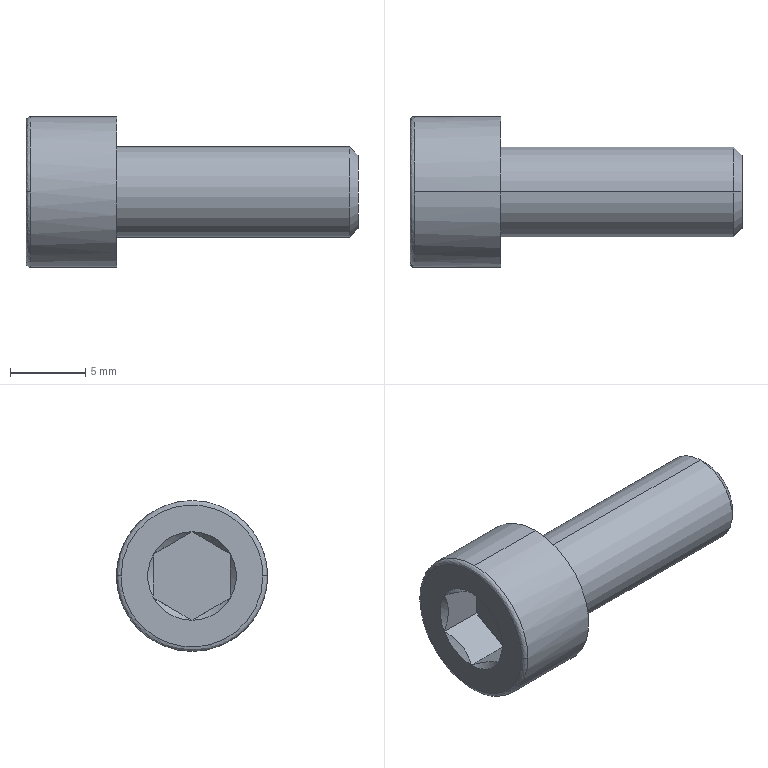Part | SolidWorks | features BaseBody 1 | 1 solid | 24 faces | box 22 x 10 x 10 mm | volume 852.514 mm3 | plane 10 | cone 8 | cylinder 4 | spline 2 | commonest cylinder face diameters 6 x2 10 x2
STEP:
#1=CARTESIAN_POINT('',(225.547,1059.506,-452.345));
#2=VERTEX_POINT('',#1);
#3=CARTESIAN_POINT('',(225.547,1050.106,-452.345));
#4=VERTEX_POINT('',#3);
#5=CARTESIAN_POINT('',(225.547,1059.506,-452.345));
#6=CARTESIAN_POINT('',(225.547,1059.506,-442.945));
#7=CARTESIAN_POINT('',(225.547,1050.106,-442.945));
#8=CARTESIAN_POINT('',(225.547,1050.106,-452.345));
#9=(BOUNDED_CURVE()B_SPLINE_CURVE(3,(#5,#6,#7,#8),.UNSPECIFIED.,.F.,.F.)B_SPLINE_CURVE_WITH_KNOTS((4,4),(0.,1.),.UNSPECIFIED.)CURVE()GEOMETRIC_REPRESENTATION_ITEM()RATIONAL_B_SPLINE_CURVE((1.,0.3333,0.3333,1.))REPRESENTATION_ITEM(''));
#10=EDGE_CURVE('',#2,#4,#9,.T.);
#11=ORIENTED_EDGE('',*,*,#10,.T.);
#12=CARTESIAN_POINT('',(225.847,1049.806,-452.345));
#13=VERTEX_POINT('',#12);
#14=CARTESIAN_POINT('',(225.847,1050.106,-452.345));
#15=DIRECTION('',(0.,0.,1.));
#16=DIRECTION('',(0.,-1.,0.));
#17=AXIS2_PLACEMENT_3D('',#14,#15,#16);
#18=CIRCLE('',#17,0.3);
#19=EDGE_CURVE('',#4,#13,#18,.T.);
#20=ORIENTED_EDGE('',*,*,#19,.T.);
#21=CARTESIAN_POINT('',(225.847,1054.806,-447.345));
#22=VERTEX_POINT('',#21);
#23=CARTESIAN_POINT('',(225.847,1054.806,-452.345));
#24=DIRECTION('',(1.,0.,0.));
#25=DIRECTION('',(0.,0.,-1.));
#26=AXIS2_PLACEMENT_3D('',#23,#24,#25);
#27=CIRCLE('',#26,5.);
#28=EDGE_CURVE('',#22,#13,#27,.T.);
#29=ORIENTED_EDGE('',*,*,#28,.F.);
#30=CARTESIAN_POINT('',(225.847,1059.806,-452.345));
#31=VERTEX_POINT('',#30);
#32=CARTESIAN_POINT('',(225.847,1054.806,-452.345));
#33=DIRECTION('',(1.,0.,0.));
#34=DIRECTION('',(0.,0.,-1.));
#35=AXIS2_PLACEMENT_3D('',#32,#33,#34);
#36=CIRCLE('',#35,5.);
#37=EDGE_CURVE('',#31,#22,#36,.T.);
#38=ORIENTED_EDGE('',*,*,#37,.F.);
#39=CARTESIAN_POINT('',(225.847,1059.506,-452.345));
#40=DIRECTION('',(0.,0.,-1.));
#41=DIRECTION('',(0.,1.,0.));
#42=AXIS2_PLACEMENT_3D('',#39,#40,#41);
#43=CIRCLE('',#42,0.3);
#44=EDGE_CURVE('',#2,#31,#43,.T.);
#45=ORIENTED_EDGE('',*,*,#44,.F.);
#46=EDGE_LOOP('',(#11,#20,#29,#38,#45));
#47=FACE_OUTER_BOUND('',#46,.T.);
#48=CARTESIAN_POINT('',(225.547,1050.106,-452.345));
#49=CARTESIAN_POINT('',(225.547,1050.106,-442.945));
#50=CARTESIAN_POINT('',(225.547,1059.506,-442.945));
#51=CARTESIAN_POINT('',(225.547,1059.506,-452.345));
#52=CARTESIAN_POINT('',(225.547,1049.93,-452.345));
#53=CARTESIAN_POINT('',(225.547,1049.93,-442.593));
#54=CARTESIAN_POINT('',(225.547,1059.681,-442.593));
#55=CARTESIAN_POINT('',(225.547,1059.681,-452.345));
#56=CARTESIAN_POINT('',(225.671,1049.806,-452.345));
#57=CARTESIAN_POINT('',(225.671,1049.806,-442.345));
#58=CARTESIAN_POINT('',(225.671,1059.806,-442.345));
#59=CARTESIAN_POINT('',(225.671,1059.806,-452.345));
#60=CARTESIAN_POINT('',(225.847,1049.806,-452.345));
#61=CARTESIAN_POINT('',(225.847,1049.806,-442.345));
#62=CARTESIAN_POINT('',(225.847,1059.806,-442.345));
#63=CARTESIAN_POINT('',(225.847,1059.806,-452.345));
#64=(BOUNDED_SURFACE()B_SPLINE_SURFACE(3,3,((#48,#49,#50,#51),(#52,#53,#54,#55),(#56,#57,#58,#59),(#60,#61,#62,#63)),.UNSPECIFIED.,.F.,.F.,.F.)B_SPLINE_SURFACE_WITH_KNOTS((4,4),(4,4),(0.,1.),(0.,1.),.UNSPECIFIED.)GEOMETRIC_REPRESENTATION_ITEM()RATIONAL_B_SPLINE_SURFACE(((1.,0.3333,0.3333,1.),(0.8047,0.2682,0.2682,0.8047),(0.8047,0.2682,0.2682,0.8047),(1.,0.3333,0.3333,1.)))REPRESENTATION_ITEM('')SURFACE());
#65=ADVANCED_FACE('',(#47),#64,.T.);
#66=CARTESIAN_POINT('',(246.992,1054.806,-449.345));
#67=VERTEX_POINT('',#66);
#68=CARTESIAN_POINT('',(246.992,1054.806,-455.345));
#69=VERTEX_POINT('',#68);
#70=CARTESIAN_POINT('',(246.992,1054.806,-452.345));
#71=DIRECTION('',(-1.,0.,0.));
#72=DIRECTION('',(0.,0.,1.));
#73=AXIS2_PLACEMENT_3D('',#70,#71,#72);
#74=CIRCLE('',#73,3.);
#75=EDGE_CURVE('',#67,#69,#74,.T.);
#76=ORIENTED_EDGE('',*,*,#75,.T.);
#77=CARTESIAN_POINT('',(231.547,1054.806,-455.345));
#78=VERTEX_POINT('',#77);
#79=CARTESIAN_POINT('',(247.547,1054.806,-455.345));
#80=DIRECTION('',(-1.,0.,0.));
#81=VECTOR('',#80,1000.);
#82=LINE('',#79,#81);
#83=EDGE_CURVE('',#69,#78,#82,.T.);
#84=ORIENTED_EDGE('',*,*,#83,.T.);
#85=CARTESIAN_POINT('',(231.547,1054.806,-449.345));
#86=VERTEX_POINT('',#85);
#87=CARTESIAN_POINT('',(231.547,1054.806,-452.345));
#88=DIRECTION('',(1.,0.,0.));
#89=DIRECTION('',(0.,0.,1.));
#90=AXIS2_PLACEMENT_3D('',#87,#88,#89);
#91=CIRCLE('',#90,3.);
#92=EDGE_CURVE('',#78,#86,#91,.T.);
#93=ORIENTED_EDGE('',*,*,#92,.T.);
#94=CARTESIAN_POINT('',(247.547,1054.806,-449.345));
#95=DIRECTION('',(-1.,0.,0.));
#96=VECTOR('',#95,1000.);
#97=LINE('',#94,#96);
#98=EDGE_CURVE('',#67,#86,#97,.T.);
#99=ORIENTED_EDGE('',*,*,#98,.F.);
#100=EDGE_LOOP('',(#76,#84,#93,#99));
#101=FACE_OUTER_BOUND('',#100,.T.);
#102=CARTESIAN_POINT('',(247.547,1054.806,-452.345));
#103=DIRECTION('',(-1.,0.,0.));
#104=DIRECTION('',(0.,0.,1.));
#105=AXIS2_PLACEMENT_3D('',#102,#103,#104);
#106=CYLINDRICAL_SURFACE('',#105,3.);
#107=ADVANCED_FACE('',(#101),#106,.T.);
#108=CARTESIAN_POINT('',(247.547,1054.806,-449.9));
#109=VERTEX_POINT('',#108);
#110=CARTESIAN_POINT('',(247.547,1054.806,-454.79));
#111=VERTEX_POINT('',#110);
#112=CARTESIAN_POINT('',(247.547,1054.806,-452.345));
#113=DIRECTION('',(-1.,0.,0.));
#114=DIRECTION('',(0.,0.,1.));
#115=AXIS2_PLACEMENT_3D('',#112,#113,#114);
#116=CIRCLE('',#115,2.445);
#117=EDGE_CURVE('',#109,#111,#116,.T.);
#118=ORIENTED_EDGE('',*,*,#117,.T.);
#119=CARTESIAN_POINT('',(246.992,1054.806,-455.345));
#120=DIRECTION('',(-0.7071,0.,-0.7071));
#121=VECTOR('',#120,1000.);
#122=LINE('',#119,#121);
#123=EDGE_CURVE('',#111,#69,#122,.T.);
#124=ORIENTED_EDGE('',*,*,#123,.T.);
#125=ORIENTED_EDGE('',*,*,#75,.F.);
#126=CARTESIAN_POINT('',(246.992,1054.806,-449.345));
#127=DIRECTION('',(-0.7071,0.,0.7071));
#128=VECTOR('',#127,1000.);
#129=LINE('',#126,#128);
#130=EDGE_CURVE('',#109,#67,#129,.T.);
#131=ORIENTED_EDGE('',*,*,#130,.F.);
#132=EDGE_LOOP('',(#118,#124,#125,#131));
#133=FACE_OUTER_BOUND('',#132,.T.);
#134=CARTESIAN_POINT('',(246.992,1054.806,-452.345));
#135=DIRECTION('',(-1.,0.,0.));
#136=DIRECTION('',(0.,0.,1.));
#137=AXIS2_PLACEMENT_3D('',#134,#135,#136);
#138=CONICAL_SURFACE('',#137,3.,0.7854);
#139=ADVANCED_FACE('',(#133),#138,.T.);
#140=CARTESIAN_POINT('',(225.847,1054.806,-457.345));
#141=VERTEX_POINT('',#140);
#142=CARTESIAN_POINT('',(225.847,1054.806,-452.345));
#143=DIRECTION('',(1.,0.,0.));
#144=DIRECTION('',(0.,0.,-1.));
#145=AXIS2_PLACEMENT_3D('',#142,#143,#144);
#146=CIRCLE('',#145,5.);
#147=EDGE_CURVE('',#141,#31,#146,.T.);
#148=ORIENTED_EDGE('',*,*,#147,.T.);
#149=ORIENTED_EDGE('',*,*,#37,.T.);
#150=CARTESIAN_POINT('',(231.547,1054.806,-447.345));
#151=VERTEX_POINT('',#150);
#152=CARTESIAN_POINT('',(225.547,1054.806,-447.345));
#153=DIRECTION('',(1.,0.,0.));
#154=VECTOR('',#153,1000.);
#155=LINE('',#152,#154);
#156=EDGE_CURVE('',#22,#151,#155,.T.);
#157=ORIENTED_EDGE('',*,*,#156,.T.);
#158=CARTESIAN_POINT('',(231.547,1054.806,-457.345));
#159=VERTEX_POINT('',#158);
#160=CARTESIAN_POINT('',(231.547,1054.806,-452.345));
#161=DIRECTION('',(-1.,0.,0.));
#162=DIRECTION('',(0.,0.,-1.));
#163=AXIS2_PLACEMENT_3D('',#160,#161,#162);
#164=CIRCLE('',#163,5.);
#165=EDGE_CURVE('',#151,#159,#164,.T.);
#166=ORIENTED_EDGE('',*,*,#165,.T.);
#167=CARTESIAN_POINT('',(225.547,1054.806,-457.345));
#168=DIRECTION('',(1.,0.,0.));
#169=VECTOR('',#168,1000.);
#170=LINE('',#167,#169);
#171=EDGE_CURVE('',#141,#159,#170,.T.);
#172=ORIENTED_EDGE('',*,*,#171,.F.);
#173=EDGE_LOOP('',(#148,#149,#157,#166,#172));
#174=FACE_OUTER_BOUND('',#173,.T.);
#175=CARTESIAN_POINT('',(225.547,1054.806,-452.345));
#176=DIRECTION('',(1.,0.,0.));
#177=DIRECTION('',(0.,0.,-1.));
#178=AXIS2_PLACEMENT_3D('',#175,#176,#177);
#179=CYLINDRICAL_SURFACE('',#178,5.);
#180=ADVANCED_FACE('',(#174),#179,.T.);
#181=ORIENTED_EDGE('',*,*,#83,.F.);
#182=CARTESIAN_POINT('',(246.992,1054.806,-452.345));
#183=DIRECTION('',(-1.,0.,0.));
#184=DIRECTION('',(0.,0.,1.));
#185=AXIS2_PLACEMENT_3D('',#182,#183,#184);
#186=CIRCLE('',#185,3.);
#187=EDGE_CURVE('',#69,#67,#186,.T.);
#188=ORIENTED_EDGE('',*,*,#187,.T.);
#189=ORIENTED_EDGE('',*,*,#98,.T.);
#190=CARTESIAN_POINT('',(231.547,1054.806,-452.345));
#191=DIRECTION('',(1.,0.,0.));
#192=DIRECTION('',(0.,0.,1.));
#193=AXIS2_PLACEMENT_3D('',#190,#191,#192);
#194=CIRCLE('',#193,3.);
#195=EDGE_CURVE('',#86,#78,#194,.T.);
#196=ORIENTED_EDGE('',*,*,#195,.T.);
#197=EDGE_LOOP('',(#181,#188,#189,#196));
#198=FACE_OUTER_BOUND('',#197,.T.);
#199=CARTESIAN_POINT('',(247.547,1054.806,-452.345));
#200=DIRECTION('',(-1.,0.,0.));
#201=DIRECTION('',(0.,0.,1.));
#202=AXIS2_PLACEMENT_3D('',#199,#200,#201);
#203=CYLINDRICAL_SURFACE('',#202,3.);
#204=ADVANCED_FACE('',(#198),#203,.T.);
#205=ORIENTED_EDGE('',*,*,#123,.F.);
#206=CARTESIAN_POINT('',(247.547,1054.806,-452.345));
#207=DIRECTION('',(-1.,0.,0.));
#208=DIRECTION('',(0.,0.,1.));
#209=AXIS2_PLACEMENT_3D('',#206,#207,#208);
#210=CIRCLE('',#209,2.445);
#211=EDGE_CURVE('',#111,#109,#210,.T.);
#212=ORIENTED_EDGE('',*,*,#211,.T.);
#213=ORIENTED_EDGE('',*,*,#130,.T.);
#214=ORIENTED_EDGE('',*,*,#187,.F.);
#215=EDGE_LOOP('',(#205,#212,#213,#214));
#216=FACE_OUTER_BOUND('',#215,.T.);
#217=CARTESIAN_POINT('',(246.992,1054.806,-452.345));
#218=DIRECTION('',(-1.,0.,0.));
#219=DIRECTION('',(0.,0.,1.));
#220=AXIS2_PLACEMENT_3D('',#217,#218,#219);
#221=CONICAL_SURFACE('',#220,3.,0.7854);
#222=ADVANCED_FACE('',(#216),#221,.T.);
#223=ORIENTED_EDGE('',*,*,#195,.F.);
#224=ORIENTED_EDGE('',*,*,#92,.F.);
#225=EDGE_LOOP('',(#223,#224));
#226=FACE_BOUND('',#225,.T.);
#227=CARTESIAN_POINT('',(231.547,1054.806,-452.345));
#228=DIRECTION('',(-1.,0.,0.));
#229=DIRECTION('',(0.,0.,-1.));
#230=AXIS2_PLACEMENT_3D('',#227,#228,#229);
#231=CIRCLE('',#230,5.);
#232=EDGE_CURVE('',#159,#151,#231,.T.);
#233=ORIENTED_EDGE('',*,*,#232,.F.);
#234=ORIENTED_EDGE('',*,*,#165,.F.);
#235=EDGE_LOOP('',(#233,#234));
#236=FACE_OUTER_BOUND('',#235,.T.);
#237=CARTESIAN_POINT('',(231.547,1054.806,-452.345));
#238=DIRECTION('',(-1.,0.,0.));
#239=DIRECTION('',(0.,0.,1.));
#240=AXIS2_PLACEMENT_3D('',#237,#238,#239);
#241=PLANE('',#240);
#242=ADVANCED_FACE('',(#226,#236),#241,.F.);
#243=ORIENTED_EDGE('',*,*,#117,.F.);
#244=ORIENTED_EDGE('',*,*,#211,.F.);
#245=EDGE_LOOP('',(#243,#244));
#246=FACE_OUTER_BOUND('',#245,.T.);
#247=CARTESIAN_POINT('',(247.547,1054.806,-452.345));
#248=DIRECTION('',(1.,0.,0.));
#249=DIRECTION('',(0.,0.,-1.));
#250=AXIS2_PLACEMENT_3D('',#247,#248,#249);
#251=PLANE('',#250);
#252=ADVANCED_FACE('',(#246),#251,.T.);
#253=ORIENTED_EDGE('',*,*,#156,.F.);
#254=ORIENTED_EDGE('',*,*,#28,.T.);
#255=CARTESIAN_POINT('',(225.847,1054.806,-452.345));
#256=DIRECTION('',(1.,0.,0.));
#257=DIRECTION('',(0.,0.,-1.));
#258=AXIS2_PLACEMENT_3D('',#255,#256,#257);
#259=CIRCLE('',#258,5.);
#260=EDGE_CURVE('',#13,#141,#259,.T.);
#261=ORIENTED_EDGE('',*,*,#260,.T.);
#262=ORIENTED_EDGE('',*,*,#171,.T.);
#263=ORIENTED_EDGE('',*,*,#232,.T.);
#264=EDGE_LOOP('',(#253,#254,#261,#262,#263));
#265=FACE_OUTER_BOUND('',#264,.T.);
#266=CARTESIAN_POINT('',(225.547,1054.806,-452.345));
#267=DIRECTION('',(1.,0.,0.));
#268=DIRECTION('',(0.,0.,-1.));
#269=AXIS2_PLACEMENT_3D('',#266,#267,#268);
#270=CYLINDRICAL_SURFACE('',#269,5.);
#271=ADVANCED_FACE('',(#265),#270,.T.);
#272=ORIENTED_EDGE('',*,*,#19,.F.);
#273=CARTESIAN_POINT('',(225.547,1050.106,-452.345));
#274=CARTESIAN_POINT('',(225.547,1050.106,-461.745));
#275=CARTESIAN_POINT('',(225.547,1059.506,-461.745));
#276=CARTESIAN_POINT('',(225.547,1059.506,-452.345));
#277=(BOUNDED_CURVE()B_SPLINE_CURVE(3,(#273,#274,#275,#276),.UNSPECIFIED.,.F.,.F.)B_SPLINE_CURVE_WITH_KNOTS((4,4),(0.,1.),.UNSPECIFIED.)CURVE()GEOMETRIC_REPRESENTATION_ITEM()RATIONAL_B_SPLINE_CURVE((1.,0.3333,0.3333,1.))REPRESENTATION_ITEM(''));
#278=EDGE_CURVE('',#4,#2,#277,.T.);
#279=ORIENTED_EDGE('',*,*,#278,.T.);
#280=ORIENTED_EDGE('',*,*,#44,.T.);
#281=ORIENTED_EDGE('',*,*,#147,.F.);
#282=ORIENTED_EDGE('',*,*,#260,.F.);
#283=EDGE_LOOP('',(#272,#279,#280,#281,#282));
#284=FACE_OUTER_BOUND('',#283,.T.);
#285=CARTESIAN_POINT('',(225.547,1059.506,-452.345));
#286=CARTESIAN_POINT('',(225.547,1059.506,-461.745));
#287=CARTESIAN_POINT('',(225.547,1050.106,-461.745));
#288=CARTESIAN_POINT('',(225.547,1050.106,-452.345));
#289=CARTESIAN_POINT('',(225.547,1059.681,-452.345));
#290=CARTESIAN_POINT('',(225.547,1059.681,-462.096));
#291=CARTESIAN_POINT('',(225.547,1049.93,-462.096));
#292=CARTESIAN_POINT('',(225.547,1049.93,-452.345));
#293=CARTESIAN_POINT('',(225.671,1059.806,-452.345));
#294=CARTESIAN_POINT('',(225.671,1059.806,-462.345));
#295=CARTESIAN_POINT('',(225.671,1049.806,-462.345));
#296=CARTESIAN_POINT('',(225.671,1049.806,-452.345));
#297=CARTESIAN_POINT('',(225.847,1059.806,-452.345));
#298=CARTESIAN_POINT('',(225.847,1059.806,-462.345));
#299=CARTESIAN_POINT('',(225.847,1049.806,-462.345));
#300=CARTESIAN_POINT('',(225.847,1049.806,-452.345));
#301=(BOUNDED_SURFACE()B_SPLINE_SURFACE(3,3,((#285,#286,#287,#288),(#289,#290,#291,#292),(#293,#294,#295,#296),(#297,#298,#299,#300)),.UNSPECIFIED.,.F.,.F.,.F.)B_SPLINE_SURFACE_WITH_KNOTS((4,4),(4,4),(0.,1.),(0.,1.),.UNSPECIFIED.)GEOMETRIC_REPRESENTATION_ITEM()RATIONAL_B_SPLINE_SURFACE(((1.,0.3333,0.3333,1.),(0.8047,0.2682,0.2682,0.8047),(0.8047,0.2682,0.2682,0.8047),(1.,0.3333,0.3333,1.)))REPRESENTATION_ITEM('')SURFACE());
#302=ADVANCED_FACE('',(#284),#301,.T.);
#303=CARTESIAN_POINT('',(225.547,1054.806,-449.412));
#304=VERTEX_POINT('',#303);
#305=CARTESIAN_POINT('',(225.547,1052.265,-450.878));
#306=VERTEX_POINT('',#305);
#307=CARTESIAN_POINT('',(225.547,1054.806,-452.345));
#308=DIRECTION('',(1.,0.,0.));
#309=DIRECTION('',(0.,0.,1.));
#310=AXIS2_PLACEMENT_3D('',#307,#308,#309);
#311=CIRCLE('',#310,2.933);
#312=EDGE_CURVE('',#304,#306,#311,.T.);
#313=ORIENTED_EDGE('',*,*,#312,.T.);
#314=CARTESIAN_POINT('',(225.547,1052.266,-453.811));
#315=VERTEX_POINT('',#314);
#316=CARTESIAN_POINT('',(225.547,1054.806,-452.345));
#317=DIRECTION('',(1.,0.,0.));
#318=DIRECTION('',(0.,0.,1.));
#319=AXIS2_PLACEMENT_3D('',#316,#317,#318);
#320=CIRCLE('',#319,2.933);
#321=EDGE_CURVE('',#306,#315,#320,.T.);
#322=ORIENTED_EDGE('',*,*,#321,.T.);
#323=CARTESIAN_POINT('',(225.547,1054.806,-455.278));
#324=VERTEX_POINT('',#323);
#325=CARTESIAN_POINT('',(225.547,1054.806,-452.345));
#326=DIRECTION('',(1.,0.,0.));
#327=DIRECTION('',(0.,0.,1.));
#328=AXIS2_PLACEMENT_3D('',#325,#326,#327);
#329=CIRCLE('',#328,2.933);
#330=EDGE_CURVE('',#315,#324,#329,.T.);
#331=ORIENTED_EDGE('',*,*,#330,.T.);
#332=CARTESIAN_POINT('',(225.547,1057.346,-453.811));
#333=VERTEX_POINT('',#332);
#334=CARTESIAN_POINT('',(225.547,1054.806,-452.345));
#335=DIRECTION('',(1.,0.,0.));
#336=DIRECTION('',(0.,0.,1.));
#337=AXIS2_PLACEMENT_3D('',#334,#335,#336);
#338=CIRCLE('',#337,2.933);
#339=EDGE_CURVE('',#324,#333,#338,.T.);
#340=ORIENTED_EDGE('',*,*,#339,.T.);
#341=CARTESIAN_POINT('',(225.547,1057.346,-450.878));
#342=VERTEX_POINT('',#341);
#343=CARTESIAN_POINT('',(225.547,1054.806,-452.345));
#344=DIRECTION('',(1.,0.,0.));
#345=DIRECTION('',(0.,0.,1.));
#346=AXIS2_PLACEMENT_3D('',#343,#344,#345);
#347=CIRCLE('',#346,2.933);
#348=EDGE_CURVE('',#333,#342,#347,.T.);
#349=ORIENTED_EDGE('',*,*,#348,.T.);
#350=CARTESIAN_POINT('',(225.547,1054.806,-452.345));
#351=DIRECTION('',(1.,0.,0.));
#352=DIRECTION('',(0.,0.,1.));
#353=AXIS2_PLACEMENT_3D('',#350,#351,#352);
#354=CIRCLE('',#353,2.933);
#355=EDGE_CURVE('',#342,#304,#354,.T.);
#356=ORIENTED_EDGE('',*,*,#355,.T.);
#357=EDGE_LOOP('',(#313,#322,#331,#340,#349,#356));
#358=FACE_BOUND('',#357,.T.);
#359=ORIENTED_EDGE('',*,*,#10,.F.);
#360=ORIENTED_EDGE('',*,*,#278,.F.);
#361=EDGE_LOOP('',(#359,#360));
#362=FACE_OUTER_BOUND('',#361,.T.);
#363=CARTESIAN_POINT('',(225.547,1054.806,-452.345));
#364=DIRECTION('',(-1.,0.,0.));
#365=DIRECTION('',(0.,0.,1.));
#366=AXIS2_PLACEMENT_3D('',#363,#364,#365);
#367=PLANE('',#366);
#368=ADVANCED_FACE('',(#358,#362),#367,.T.);
#369=CARTESIAN_POINT('',(225.547,1052.266,-453.811));
#370=CARTESIAN_POINT('',(225.661,1052.266,-453.582));
#371=CARTESIAN_POINT('',(225.758,1052.266,-453.348));
#372=CARTESIAN_POINT('',(225.898,1052.266,-452.863));
#373=CARTESIAN_POINT('',(225.939,1052.266,-452.609));
#374=CARTESIAN_POINT('',(225.94,1052.266,-452.092));
#375=CARTESIAN_POINT('',(225.901,1052.266,-451.84));
#376=CARTESIAN_POINT('',(225.761,1052.266,-451.348));
#377=CARTESIAN_POINT('',(225.662,1052.266,-451.108));
#378=CARTESIAN_POINT('',(225.547,1052.265,-450.878));
#379=B_SPLINE_CURVE_WITH_KNOTS('',3,(#369,#370,#371,#372,#373,#374,#375,#376,#377,#378),.UNSPECIFIED.,.F.,.F.,(4,2,2,2,4),(0.,0.0007567,0.001513,0.00227,0.003027),.UNSPECIFIED.);
#380=EDGE_CURVE('',#315,#306,#379,.T.);
#381=ORIENTED_EDGE('',*,*,#380,.F.);
#382=ORIENTED_EDGE('',*,*,#321,.F.);
#383=EDGE_LOOP('',(#381,#382));
#384=FACE_OUTER_BOUND('',#383,.T.);
#385=CARTESIAN_POINT('',(225.544,1054.806,-452.345));
#386=DIRECTION('',(-1.,0.,0.));
#387=DIRECTION('',(0.,0.,1.));
#388=AXIS2_PLACEMENT_3D('',#385,#386,#387);
#389=CONICAL_SURFACE('',#388,2.935,0.7854);
#390=ADVANCED_FACE('',(#384),#389,.F.);
#391=CARTESIAN_POINT('',(225.547,1052.265,-450.878));
#392=CARTESIAN_POINT('',(225.661,1052.464,-450.764));
#393=CARTESIAN_POINT('',(225.759,1052.667,-450.646));
#394=CARTESIAN_POINT('',(225.863,1052.982,-450.464));
#395=CARTESIAN_POINT('',(225.891,1053.089,-450.403));
#396=CARTESIAN_POINT('',(225.929,1053.307,-450.277));
#397=CARTESIAN_POINT('',(225.939,1053.42,-450.212));
#398=CARTESIAN_POINT('',(225.94,1053.753,-450.02));
#399=CARTESIAN_POINT('',(225.901,1053.971,-449.894));
#400=CARTESIAN_POINT('',(225.761,1054.4,-449.646));
#401=CARTESIAN_POINT('',(225.662,1054.606,-449.527));
#402=CARTESIAN_POINT('',(225.547,1054.806,-449.412));
#403=B_SPLINE_CURVE_WITH_KNOTS('',3,(#391,#392,#393,#394,#395,#396,#397,#398,#399,#400,#401,#402),.UNSPECIFIED.,.F.,.F.,(4,2,2,2,2,4),(0.,0.0007574,0.001136,0.001515,0.002272,0.00303),.UNSPECIFIED.);
#404=EDGE_CURVE('',#306,#304,#403,.T.);
#405=ORIENTED_EDGE('',*,*,#404,.F.);
#406=ORIENTED_EDGE('',*,*,#312,.F.);
#407=EDGE_LOOP('',(#405,#406));
#408=FACE_OUTER_BOUND('',#407,.T.);
#409=CARTESIAN_POINT('',(225.547,1054.806,-452.345));
#410=DIRECTION('',(-1.,0.,0.));
#411=DIRECTION('',(0.,0.,1.));
#412=AXIS2_PLACEMENT_3D('',#409,#410,#411);
#413=CONICAL_SURFACE('',#412,2.933,0.7854);
#414=ADVANCED_FACE('',(#408),#413,.F.);
#415=CARTESIAN_POINT('',(225.547,1054.806,-449.412));
#416=CARTESIAN_POINT('',(225.661,1055.004,-449.526));
#417=CARTESIAN_POINT('',(225.759,1055.207,-449.643));
#418=CARTESIAN_POINT('',(225.863,1055.522,-449.825));
#419=CARTESIAN_POINT('',(225.891,1055.629,-449.887));
#420=CARTESIAN_POINT('',(225.929,1055.848,-450.013));
#421=CARTESIAN_POINT('',(225.939,1055.96,-450.078));
#422=CARTESIAN_POINT('',(225.94,1056.293,-450.27));
#423=CARTESIAN_POINT('',(225.901,1056.511,-450.396));
#424=CARTESIAN_POINT('',(225.761,1056.94,-450.644));
#425=CARTESIAN_POINT('',(225.662,1057.146,-450.763));
#426=CARTESIAN_POINT('',(225.547,1057.346,-450.878));
#427=B_SPLINE_CURVE_WITH_KNOTS('',3,(#415,#416,#417,#418,#419,#420,#421,#422,#423,#424,#425,#426),.UNSPECIFIED.,.F.,.F.,(4,2,2,2,2,4),(0.,0.0007574,0.001136,0.001515,0.002272,0.00303),.UNSPECIFIED.);
#428=EDGE_CURVE('',#304,#342,#427,.T.);
#429=ORIENTED_EDGE('',*,*,#428,.F.);
#430=ORIENTED_EDGE('',*,*,#355,.F.);
#431=EDGE_LOOP('',(#429,#430));
#432=FACE_OUTER_BOUND('',#431,.T.);
#433=CARTESIAN_POINT('',(225.547,1054.806,-452.345));
#434=DIRECTION('',(-1.,0.,0.));
#435=DIRECTION('',(0.,0.,1.));
#436=AXIS2_PLACEMENT_3D('',#433,#434,#435);
#437=CONICAL_SURFACE('',#436,2.933,0.7854);
#438=ADVANCED_FACE('',(#432),#437,.F.);
#439=CARTESIAN_POINT('',(225.547,1057.346,-450.878));
#440=CARTESIAN_POINT('',(225.661,1057.346,-451.107));
#441=CARTESIAN_POINT('',(225.758,1057.346,-451.341));
#442=CARTESIAN_POINT('',(225.898,1057.346,-451.826));
#443=CARTESIAN_POINT('',(225.939,1057.346,-452.08));
#444=CARTESIAN_POINT('',(225.94,1057.346,-452.597));
#445=CARTESIAN_POINT('',(225.901,1057.346,-452.849));
#446=CARTESIAN_POINT('',(225.761,1057.346,-453.342));
#447=CARTESIAN_POINT('',(225.662,1057.346,-453.581));
#448=CARTESIAN_POINT('',(225.547,1057.346,-453.811));
#449=B_SPLINE_CURVE_WITH_KNOTS('',3,(#439,#440,#441,#442,#443,#444,#445,#446,#447,#448),.UNSPECIFIED.,.F.,.F.,(4,2,2,2,4),(0.,0.0007567,0.001513,0.00227,0.003027),.UNSPECIFIED.);
#450=EDGE_CURVE('',#342,#333,#449,.T.);
#451=ORIENTED_EDGE('',*,*,#450,.F.);
#452=ORIENTED_EDGE('',*,*,#348,.F.);
#453=EDGE_LOOP('',(#451,#452));
#454=FACE_OUTER_BOUND('',#453,.T.);
#455=CARTESIAN_POINT('',(225.544,1054.806,-452.345));
#456=DIRECTION('',(-1.,0.,0.));
#457=DIRECTION('',(0.,0.,1.));
#458=AXIS2_PLACEMENT_3D('',#455,#456,#457);
#459=CONICAL_SURFACE('',#458,2.935,0.7854);
#460=ADVANCED_FACE('',(#454),#459,.F.);
#461=CARTESIAN_POINT('',(225.547,1057.346,-453.811));
#462=CARTESIAN_POINT('',(225.661,1057.147,-453.926));
#463=CARTESIAN_POINT('',(225.759,1056.944,-454.043));
#464=CARTESIAN_POINT('',(225.863,1056.629,-454.225));
#465=CARTESIAN_POINT('',(225.891,1056.522,-454.287));
#466=CARTESIAN_POINT('',(225.929,1056.304,-454.413));
#467=CARTESIAN_POINT('',(225.939,1056.191,-454.478));
#468=CARTESIAN_POINT('',(225.94,1055.858,-454.67));
#469=CARTESIAN_POINT('',(225.901,1055.641,-454.795));
#470=CARTESIAN_POINT('',(225.761,1055.211,-455.044));
#471=CARTESIAN_POINT('',(225.662,1055.005,-455.162));
#472=CARTESIAN_POINT('',(225.547,1054.806,-455.278));
#473=B_SPLINE_CURVE_WITH_KNOTS('',3,(#461,#462,#463,#464,#465,#466,#467,#468,#469,#470,#471,#472),.UNSPECIFIED.,.F.,.F.,(4,2,2,2,2,4),(0.,0.0007574,0.001136,0.001515,0.002272,0.00303),.UNSPECIFIED.);
#474=EDGE_CURVE('',#333,#324,#473,.T.);
#475=ORIENTED_EDGE('',*,*,#474,.F.);
#476=ORIENTED_EDGE('',*,*,#339,.F.);
#477=EDGE_LOOP('',(#475,#476));
#478=FACE_OUTER_BOUND('',#477,.T.);
#479=CARTESIAN_POINT('',(225.547,1054.806,-452.345));
#480=DIRECTION('',(-1.,0.,0.));
#481=DIRECTION('',(0.,0.,1.));
#482=AXIS2_PLACEMENT_3D('',#479,#480,#481);
#483=CONICAL_SURFACE('',#482,2.933,0.7854);
#484=ADVANCED_FACE('',(#478),#483,.F.);
#485=CARTESIAN_POINT('',(225.547,1054.806,-455.278));
#486=CARTESIAN_POINT('',(225.661,1054.607,-455.163));
#487=CARTESIAN_POINT('',(225.759,1054.404,-455.046));
#488=CARTESIAN_POINT('',(225.863,1054.089,-454.864));
#489=CARTESIAN_POINT('',(225.891,1053.982,-454.802));
#490=CARTESIAN_POINT('',(225.929,1053.764,-454.676));
#491=CARTESIAN_POINT('',(225.939,1053.651,-454.611));
#492=CARTESIAN_POINT('',(225.94,1053.318,-454.419));
#493=CARTESIAN_POINT('',(225.901,1053.101,-454.293));
#494=CARTESIAN_POINT('',(225.761,1052.671,-454.045));
#495=CARTESIAN_POINT('',(225.662,1052.465,-453.926));
#496=CARTESIAN_POINT('',(225.547,1052.266,-453.811));
#497=B_SPLINE_CURVE_WITH_KNOTS('',3,(#485,#486,#487,#488,#489,#490,#491,#492,#493,#494,#495,#496),.UNSPECIFIED.,.F.,.F.,(4,2,2,2,2,4),(0.,0.0007574,0.001136,0.001515,0.002272,0.00303),.UNSPECIFIED.);
#498=EDGE_CURVE('',#324,#315,#497,.T.);
#499=ORIENTED_EDGE('',*,*,#498,.F.);
#500=ORIENTED_EDGE('',*,*,#330,.F.);
#501=EDGE_LOOP('',(#499,#500));
#502=FACE_OUTER_BOUND('',#501,.T.);
#503=CARTESIAN_POINT('',(225.547,1054.806,-452.345));
#504=DIRECTION('',(-1.,0.,0.));
#505=DIRECTION('',(0.,0.,1.));
#506=AXIS2_PLACEMENT_3D('',#503,#504,#505);
#507=CONICAL_SURFACE('',#506,2.933,0.7854);
#508=ADVANCED_FACE('',(#502),#507,.F.);
#509=CARTESIAN_POINT('',(228.547,1052.266,-450.878));
#510=VERTEX_POINT('',#509);
#511=CARTESIAN_POINT('',(228.547,1052.266,-450.878));
#512=DIRECTION('',(-1.,0.,0.));
#513=VECTOR('',#512,1000.);
#514=LINE('',#511,#513);
#515=EDGE_CURVE('',#510,#306,#514,.T.);
#516=ORIENTED_EDGE('',*,*,#515,.F.);
#517=CARTESIAN_POINT('',(228.547,1052.266,-453.811));
#518=VERTEX_POINT('',#517);
#519=CARTESIAN_POINT('',(228.547,1052.266,-453.811));
#520=DIRECTION('',(0.,0.,1.));
#521=VECTOR('',#520,1000.);
#522=LINE('',#519,#521);
#523=EDGE_CURVE('',#518,#510,#522,.T.);
#524=ORIENTED_EDGE('',*,*,#523,.F.);
#525=CARTESIAN_POINT('',(228.547,1052.266,-453.811));
#526=DIRECTION('',(1.,0.,0.));
#527=VECTOR('',#526,1000.);
#528=LINE('',#525,#527);
#529=EDGE_CURVE('',#315,#518,#528,.T.);
#530=ORIENTED_EDGE('',*,*,#529,.F.);
#531=ORIENTED_EDGE('',*,*,#380,.T.);
#532=EDGE_LOOP('',(#516,#524,#530,#531));
#533=FACE_OUTER_BOUND('',#532,.T.);
#534=CARTESIAN_POINT('',(228.547,1052.266,-453.811));
#535=DIRECTION('',(0.,-1.,0.));
#536=DIRECTION('',(0.,0.,-1.));
#537=AXIS2_PLACEMENT_3D('',#534,#535,#536);
#538=PLANE('',#537);
#539=ADVANCED_FACE('',(#533),#538,.F.);
#540=CARTESIAN_POINT('',(228.547,1054.806,-449.412));
#541=VERTEX_POINT('',#540);
#542=CARTESIAN_POINT('',(228.547,1052.266,-450.878));
#543=DIRECTION('',(0.,0.866,0.5));
#544=VECTOR('',#543,1000.);
#545=LINE('',#542,#544);
#546=EDGE_CURVE('',#510,#541,#545,.T.);
#547=ORIENTED_EDGE('',*,*,#546,.F.);
#548=ORIENTED_EDGE('',*,*,#515,.T.);
#549=ORIENTED_EDGE('',*,*,#404,.T.);
#550=CARTESIAN_POINT('',(228.547,1054.806,-449.412));
#551=DIRECTION('',(-1.,0.,0.));
#552=VECTOR('',#551,1000.);
#553=LINE('',#550,#552);
#554=EDGE_CURVE('',#541,#304,#553,.T.);
#555=ORIENTED_EDGE('',*,*,#554,.F.);
#556=EDGE_LOOP('',(#547,#548,#549,#555));
#557=FACE_OUTER_BOUND('',#556,.T.);
#558=CARTESIAN_POINT('',(228.547,1052.266,-450.878));
#559=DIRECTION('',(0.,-0.5,0.866));
#560=DIRECTION('',(0.,-0.866,-0.5));
#561=AXIS2_PLACEMENT_3D('',#558,#559,#560);
#562=PLANE('',#561);
#563=ADVANCED_FACE('',(#557),#562,.F.);
#564=CARTESIAN_POINT('',(228.547,1057.346,-450.878));
#565=VERTEX_POINT('',#564);
#566=CARTESIAN_POINT('',(228.547,1054.806,-449.412));
#567=DIRECTION('',(0.,0.866,-0.5));
#568=VECTOR('',#567,1000.);
#569=LINE('',#566,#568);
#570=EDGE_CURVE('',#541,#565,#569,.T.);
#571=ORIENTED_EDGE('',*,*,#570,.F.);
#572=ORIENTED_EDGE('',*,*,#554,.T.);
#573=ORIENTED_EDGE('',*,*,#428,.T.);
#574=CARTESIAN_POINT('',(228.547,1057.346,-450.878));
#575=DIRECTION('',(-1.,0.,0.));
#576=VECTOR('',#575,1000.);
#577=LINE('',#574,#576);
#578=EDGE_CURVE('',#565,#342,#577,.T.);
#579=ORIENTED_EDGE('',*,*,#578,.F.);
#580=EDGE_LOOP('',(#571,#572,#573,#579));
#581=FACE_OUTER_BOUND('',#580,.T.);
#582=CARTESIAN_POINT('',(228.547,1054.806,-449.412));
#583=DIRECTION('',(0.,0.5,0.866));
#584=DIRECTION('',(0.,-0.866,0.5));
#585=AXIS2_PLACEMENT_3D('',#582,#583,#584);
#586=PLANE('',#585);
#587=ADVANCED_FACE('',(#581),#586,.F.);
#588=CARTESIAN_POINT('',(228.547,1057.346,-453.811));
#589=VERTEX_POINT('',#588);
#590=CARTESIAN_POINT('',(228.547,1057.346,-453.811));
#591=DIRECTION('',(-1.,0.,0.));
#592=VECTOR('',#591,1000.);
#593=LINE('',#590,#592);
#594=EDGE_CURVE('',#589,#333,#593,.T.);
#595=ORIENTED_EDGE('',*,*,#594,.F.);
#596=CARTESIAN_POINT('',(228.547,1057.346,-450.878));
#597=DIRECTION('',(0.,0.,-1.));
#598=VECTOR('',#597,1000.);
#599=LINE('',#596,#598);
#600=EDGE_CURVE('',#565,#589,#599,.T.);
#601=ORIENTED_EDGE('',*,*,#600,.F.);
#602=ORIENTED_EDGE('',*,*,#578,.T.);
#603=ORIENTED_EDGE('',*,*,#450,.T.);
#604=EDGE_LOOP('',(#595,#601,#602,#603));
#605=FACE_OUTER_BOUND('',#604,.T.);
#606=CARTESIAN_POINT('',(228.547,1057.346,-450.878));
#607=DIRECTION('',(0.,1.,0.));
#608=DIRECTION('',(0.,0.,1.));
#609=AXIS2_PLACEMENT_3D('',#606,#607,#608);
#610=PLANE('',#609);
#611=ADVANCED_FACE('',(#605),#610,.F.);
#612=CARTESIAN_POINT('',(228.547,1054.806,-455.278));
#613=VERTEX_POINT('',#612);
#614=CARTESIAN_POINT('',(228.547,1057.346,-453.811));
#615=DIRECTION('',(0.,-0.866,-0.5));
#616=VECTOR('',#615,1000.);
#617=LINE('',#614,#616);
#618=EDGE_CURVE('',#589,#613,#617,.T.);
#619=ORIENTED_EDGE('',*,*,#618,.F.);
#620=ORIENTED_EDGE('',*,*,#594,.T.);
#621=ORIENTED_EDGE('',*,*,#474,.T.);
#622=CARTESIAN_POINT('',(228.547,1054.806,-455.278));
#623=DIRECTION('',(-1.,0.,0.));
#624=VECTOR('',#623,1000.);
#625=LINE('',#622,#624);
#626=EDGE_CURVE('',#613,#324,#625,.T.);
#627=ORIENTED_EDGE('',*,*,#626,.F.);
#628=EDGE_LOOP('',(#619,#620,#621,#627));
#629=FACE_OUTER_BOUND('',#628,.T.);
#630=CARTESIAN_POINT('',(228.547,1057.346,-453.811));
#631=DIRECTION('',(0.,0.5,-0.866));
#632=DIRECTION('',(0.,0.866,0.5));
#633=AXIS2_PLACEMENT_3D('',#630,#631,#632);
#634=PLANE('',#633);
#635=ADVANCED_FACE('',(#629),#634,.F.);
#636=CARTESIAN_POINT('',(228.547,1054.806,-455.278));
#637=DIRECTION('',(0.,-0.866,0.5));
#638=VECTOR('',#637,1000.);
#639=LINE('',#636,#638);
#640=EDGE_CURVE('',#613,#518,#639,.T.);
#641=ORIENTED_EDGE('',*,*,#640,.F.);
#642=ORIENTED_EDGE('',*,*,#626,.T.);
#643=ORIENTED_EDGE('',*,*,#498,.T.);
#644=ORIENTED_EDGE('',*,*,#529,.T.);
#645=EDGE_LOOP('',(#641,#642,#643,#644));
#646=FACE_OUTER_BOUND('',#645,.T.);
#647=CARTESIAN_POINT('',(228.547,1054.806,-455.278));
#648=DIRECTION('',(0.,-0.5,-0.866));
#649=DIRECTION('',(0.,0.866,-0.5));
#650=AXIS2_PLACEMENT_3D('',#647,#648,#649);
#651=PLANE('',#650);
#652=ADVANCED_FACE('',(#646),#651,.F.);
#653=ORIENTED_EDGE('',*,*,#600,.T.);
#654=ORIENTED_EDGE('',*,*,#618,.T.);
#655=ORIENTED_EDGE('',*,*,#640,.T.);
#656=ORIENTED_EDGE('',*,*,#523,.T.);
#657=ORIENTED_EDGE('',*,*,#546,.T.);
#658=ORIENTED_EDGE('',*,*,#570,.T.);
#659=EDGE_LOOP('',(#653,#654,#655,#656,#657,#658));
#660=FACE_OUTER_BOUND('',#659,.T.);
#661=CARTESIAN_POINT('',(228.547,1054.806,-452.345));
#662=DIRECTION('',(-1.,0.,0.));
#663=DIRECTION('',(0.,0.,1.));
#664=AXIS2_PLACEMENT_3D('',#661,#662,#663);
#665=PLANE('',#664);
#666=ADVANCED_FACE('',(#660),#665,.T.);
#667=CLOSED_SHELL('',(#65,#107,#139,#180,#204,#222,#242,#252,#271,#302,#368,#390,#414,#438,#460,#484,#508,#539,#563,#587,#611,#635,#652,#666));
#668=MANIFOLD_SOLID_BREP('',#667);
#669=CARTESIAN_POINT('',(0.,0.,0.));
#670=DIRECTION('',(0.,0.,1.));
#671=DIRECTION('',(1.,0.,0.));
#672=AXIS2_PLACEMENT_3D('',#669,#670,#671);
#673=(LENGTH_UNIT()NAMED_UNIT(*)SI_UNIT(.MILLI.,.METRE.));
#674=UNCERTAINTY_MEASURE_WITH_UNIT(LENGTH_MEASURE(0.00001),#673,'','');
#675=(NAMED_UNIT(*)PLANE_ANGLE_UNIT()SI_UNIT($,.RADIAN.));
#676=(NAMED_UNIT(*)SI_UNIT($,.STERADIAN.)SOLID_ANGLE_UNIT());
#677=(GEOMETRIC_REPRESENTATION_CONTEXT(3)GLOBAL_UNCERTAINTY_ASSIGNED_CONTEXT((#674))GLOBAL_UNIT_ASSIGNED_CONTEXT((#673,#675,#676))REPRESENTATION_CONTEXT('',''));
#678=ADVANCED_BREP_SHAPE_REPRESENTATION('',(#668,#672),#677);